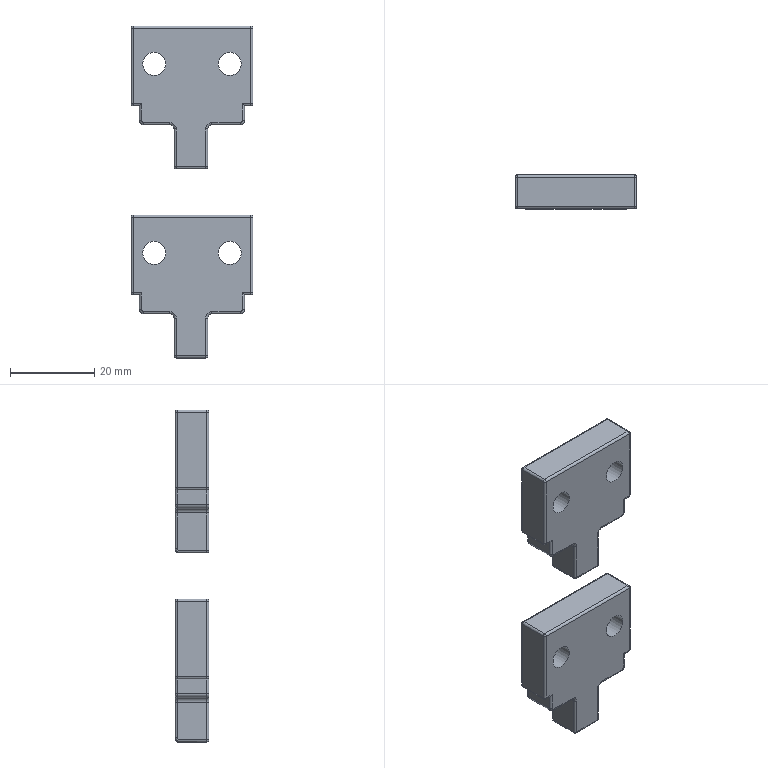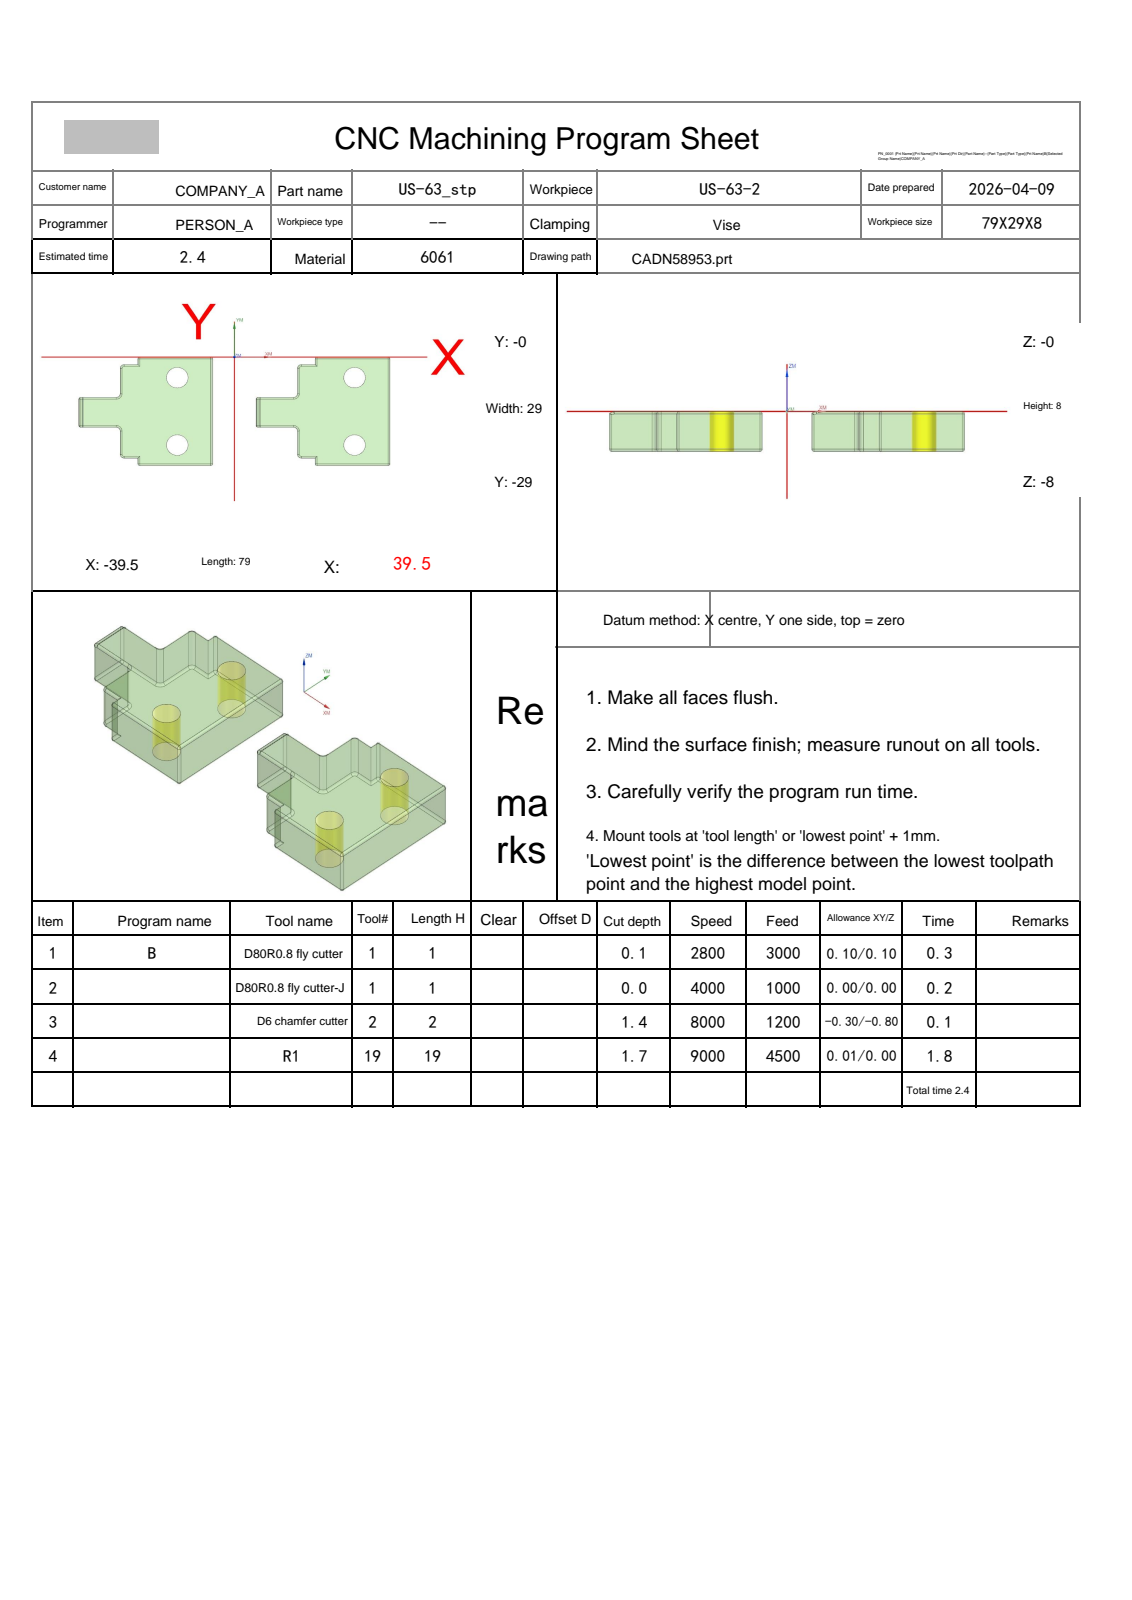NC program | NX | posted by the shop | part box 29 x 8 x 79 mm
Lines 1 to 128 of 19198:
%
O0001
(Machine time: 3.13 MIN)
(===Total Tool:3===)
(T1=D80R0.8 fly cutter D=80.  R=0.8  D-  H01 Z=0.    )
(T2=D6 chamfer cutter   D=6.   R=0.   D-  H02 Z=-1.4  )
(T19=R1     D=2.   R=1.   D-  H19 Z=-1.67 )
G80 G90 G17 G49 G40
G91 G28 Z0
M01
N1 T01 M06
(D80R0.8 fly cutter  D=80. R=0.8 H=01 ce=0.10 di=0.10)
G00 G90 G54 X91.597 Y-14.5 M03 S2800
G43 H01 Z20.
M08
Z3.525
G01 Z1.525 F3000.
X79.597
X-79.597
X-91.597
Z3.525
G00 X91.597
Z3.05
G01 Z1.05
X79.597
X-79.597
X-91.597
Z3.05
G00 X91.597
Z2.575
G01 Z.575
X79.597
X-79.597
X-91.597
Z2.575
G00 X91.597
Z2.1
G01 Z.1
X79.597
X-79.597
X-91.597
Z2.1
G00 Z20.
G91 G28 Z0.0
M05
M09
G91 G28 Z0.0
M01
N2 T01 M06
(D80R0.8 fly cutter-J  D=80. R=0.8 H=01 ce=0.00 di=0.00)
G00 G90 G54 X91.499 Y-14.5 M03 S4000
G43 H01 Z20.
M08
Z2.
G01 Z0.0 F1000.
X79.499
X-79.499
X-91.499
Z2.
G00 Z20.
G91 G28 Z0.0
M05
M09
G91 G28 Z0.0
M01
N3 T02 M06
(D6 chamfer cutter  D=6. R=0. H=02 ce=-0.30 di=-0.80)
G00 G90 G54 X30.565 Y-6.147 M03 S8000
G43 H02 Z20.
M08
Z-.9
G01 Z-1.4 F1200.
X30.65 Y-7.
G03 X32.15 Y-5.5 I0.0 J1.5
X30.5 Y-3.85 I-1.65 J0.0
X28.85 Y-5.5 I0.0 J-1.65
X30.5 Y-7.15 I1.65 J0.0
X32.15 Y-5.5 I0.0 J1.65
X30.65 Y-4. I-1.5 J0.0
G01 X30.565 Y-4.853
Z-.9
G00 Z20.
Y-24.147
Z-.9
G01 Z-1.4
X30.65 Y-25.
G03 X32.15 Y-23.5 I0.0 J1.5
X30.5 Y-21.85 I-1.65 J0.0
X28.85 Y-23.5 I0.0 J-1.65
X30.5 Y-25.15 I1.65 J0.0
X32.15 Y-23.5 I0.0 J1.65
X30.65 Y-22. I-1.5 J0.0
G01 X30.565 Y-22.853
Z-.9
G00 Z20.
X-14.435 Y-24.147
Z-.9
G01 Z-1.4
X-14.35 Y-25.
G03 X-12.85 Y-23.5 I0.0 J1.5
X-14.5 Y-21.85 I-1.65 J0.0
X-16.15 Y-23.5 I0.0 J-1.65
X-14.5 Y-25.15 I1.65 J0.0
X-12.85 Y-23.5 I0.0 J1.65
X-14.35 Y-22. I-1.5 J0.0
G01 X-14.435 Y-22.853
Z-.9
G00 Z20.
Y-6.147
Z-.9
G01 Z-1.4
X-14.35 Y-7.
G03 X-12.85 Y-5.5 I0.0 J1.5
X-14.5 Y-3.85 I-1.65 J0.0
X-16.15 Y-5.5 I0.0 J-1.65
X-14.5 Y-7.15 I1.65 J0.0
X-12.85 Y-5.5 I0.0 J1.65
X-14.35 Y-4. I-1.5 J0.0
G01 X-14.435 Y-4.853
Z-.9
G00 Z20.
G91 G28 Z0.0
M05
M09
G91 G28 Z0.0
M01